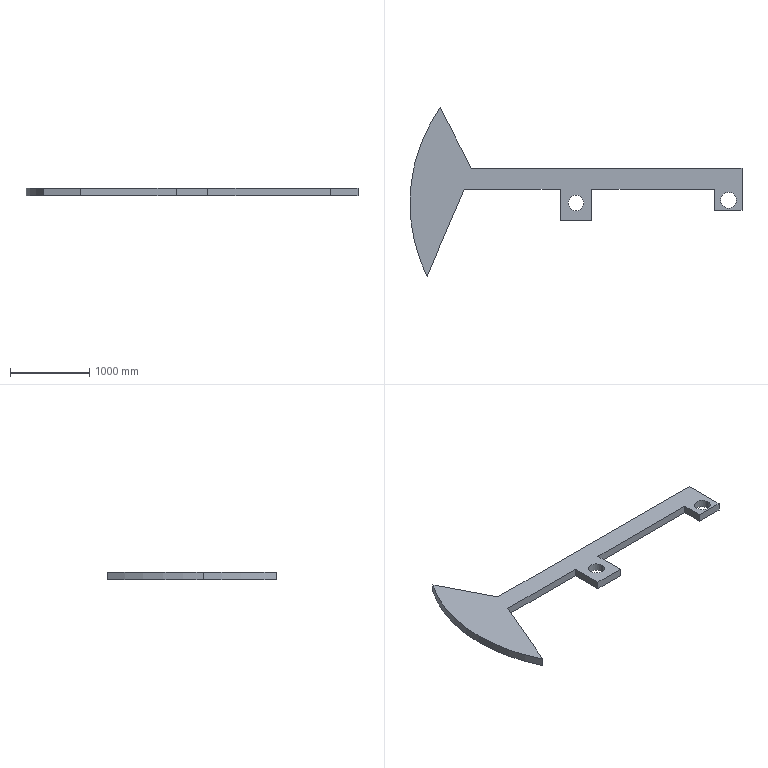Part | SolidWorks | features Extrusion 1, ICE 1 | 1 solid | 19 faces | box 4200 x 2133 x 100 mm | volume 203520372 mm3 | plane 13 | cylinder 6 | commonest cylinder face diameters 200 x4 4200 x2
STEP:
#1=CARTESIAN_POINT('',(-100.,0.,0.));
#2=VERTEX_POINT('',#1);
#3=CARTESIAN_POINT('',(100.,0.,0.));
#4=VERTEX_POINT('',#3);
#5=CARTESIAN_POINT('',(0.,0.,0.));
#6=DIRECTION('',(0.,0.,1.));
#7=DIRECTION('',(1.,0.,0.));
#8=AXIS2_PLACEMENT_3D('',#5,#6,#7);
#9=CIRCLE('',#8,100.);
#10=EDGE_CURVE('',#2,#4,#9,.T.);
#11=ORIENTED_EDGE('',*,*,#10,.F.);
#12=CARTESIAN_POINT('',(-100.,0.,100.));
#13=VERTEX_POINT('',#12);
#14=CARTESIAN_POINT('',(-100.,0.,0.));
#15=DIRECTION('',(0.,0.,1.));
#16=VECTOR('',#15,1000.);
#17=LINE('',#14,#16);
#18=EDGE_CURVE('',#2,#13,#17,.T.);
#19=ORIENTED_EDGE('',*,*,#18,.T.);
#20=CARTESIAN_POINT('',(100.,0.,100.));
#21=VERTEX_POINT('',#20);
#22=CARTESIAN_POINT('',(0.,0.,100.));
#23=DIRECTION('',(0.,0.,1.));
#24=DIRECTION('',(1.,0.,0.));
#25=AXIS2_PLACEMENT_3D('',#22,#23,#24);
#26=CIRCLE('',#25,100.);
#27=EDGE_CURVE('',#13,#21,#26,.T.);
#28=ORIENTED_EDGE('',*,*,#27,.T.);
#29=CARTESIAN_POINT('',(100.,0.,0.));
#30=DIRECTION('',(0.,0.,1.));
#31=VECTOR('',#30,1000.);
#32=LINE('',#29,#31);
#33=EDGE_CURVE('',#4,#21,#32,.T.);
#34=ORIENTED_EDGE('',*,*,#33,.F.);
#35=EDGE_LOOP('',(#11,#19,#28,#34));
#36=FACE_OUTER_BOUND('',#35,.T.);
#37=CARTESIAN_POINT('',(0.,0.,0.));
#38=DIRECTION('',(0.,0.,1.));
#39=DIRECTION('',(1.,0.,0.));
#40=AXIS2_PLACEMENT_3D('',#37,#38,#39);
#41=CYLINDRICAL_SURFACE('',#40,100.);
#42=ADVANCED_FACE('',(#36),#41,.F.);
#43=CARTESIAN_POINT('',(1830.038,35.754,0.));
#44=VERTEX_POINT('',#43);
#45=CARTESIAN_POINT('',(2030.038,35.754,0.));
#46=VERTEX_POINT('',#45);
#47=CARTESIAN_POINT('',(1930.038,35.754,0.));
#48=DIRECTION('',(0.,0.,1.));
#49=DIRECTION('',(1.,0.,0.));
#50=AXIS2_PLACEMENT_3D('',#47,#48,#49);
#51=CIRCLE('',#50,100.);
#52=EDGE_CURVE('',#44,#46,#51,.T.);
#53=ORIENTED_EDGE('',*,*,#52,.F.);
#54=CARTESIAN_POINT('',(1830.038,35.754,100.));
#55=VERTEX_POINT('',#54);
#56=CARTESIAN_POINT('',(1830.038,35.754,0.));
#57=DIRECTION('',(0.,0.,1.));
#58=VECTOR('',#57,1000.);
#59=LINE('',#56,#58);
#60=EDGE_CURVE('',#44,#55,#59,.T.);
#61=ORIENTED_EDGE('',*,*,#60,.T.);
#62=CARTESIAN_POINT('',(2030.038,35.754,100.));
#63=VERTEX_POINT('',#62);
#64=CARTESIAN_POINT('',(1930.038,35.754,100.));
#65=DIRECTION('',(0.,0.,1.));
#66=DIRECTION('',(1.,0.,0.));
#67=AXIS2_PLACEMENT_3D('',#64,#65,#66);
#68=CIRCLE('',#67,100.);
#69=EDGE_CURVE('',#55,#63,#68,.T.);
#70=ORIENTED_EDGE('',*,*,#69,.T.);
#71=CARTESIAN_POINT('',(2030.038,35.754,0.));
#72=DIRECTION('',(0.,0.,1.));
#73=VECTOR('',#72,1000.);
#74=LINE('',#71,#73);
#75=EDGE_CURVE('',#46,#63,#74,.T.);
#76=ORIENTED_EDGE('',*,*,#75,.F.);
#77=EDGE_LOOP('',(#53,#61,#70,#76));
#78=FACE_OUTER_BOUND('',#77,.T.);
#79=CARTESIAN_POINT('',(1930.038,35.754,0.));
#80=DIRECTION('',(0.,0.,1.));
#81=DIRECTION('',(1.,0.,0.));
#82=AXIS2_PLACEMENT_3D('',#79,#80,#81);
#83=CYLINDRICAL_SURFACE('',#82,100.);
#84=ADVANCED_FACE('',(#78),#83,.F.);
#85=CARTESIAN_POINT('',(-2100.,0.,100.));
#86=VERTEX_POINT('',#85);
#87=CARTESIAN_POINT('',(-1884.738,-926.156,100.));
#88=VERTEX_POINT('',#87);
#89=CARTESIAN_POINT('',(0.,0.,100.));
#90=DIRECTION('',(0.,0.,1.));
#91=DIRECTION('',(1.,0.,0.));
#92=AXIS2_PLACEMENT_3D('',#89,#90,#91);
#93=CIRCLE('',#92,2100.);
#94=EDGE_CURVE('',#86,#88,#93,.T.);
#95=ORIENTED_EDGE('',*,*,#94,.F.);
#96=CARTESIAN_POINT('',(-2100.,0.,0.));
#97=VERTEX_POINT('',#96);
#98=CARTESIAN_POINT('',(-2100.,0.,100.));
#99=DIRECTION('',(0.,0.,-1.));
#100=VECTOR('',#99,1000.);
#101=LINE('',#98,#100);
#102=EDGE_CURVE('',#86,#97,#101,.T.);
#103=ORIENTED_EDGE('',*,*,#102,.T.);
#104=CARTESIAN_POINT('',(-1884.738,-926.156,0.));
#105=VERTEX_POINT('',#104);
#106=CARTESIAN_POINT('',(0.,0.,0.));
#107=DIRECTION('',(0.,0.,1.));
#108=DIRECTION('',(1.,0.,0.));
#109=AXIS2_PLACEMENT_3D('',#106,#107,#108);
#110=CIRCLE('',#109,2100.);
#111=EDGE_CURVE('',#97,#105,#110,.T.);
#112=ORIENTED_EDGE('',*,*,#111,.T.);
#113=CARTESIAN_POINT('',(-1884.738,-926.156,100.));
#114=DIRECTION('',(0.,0.,-1.));
#115=VECTOR('',#114,1000.);
#116=LINE('',#113,#115);
#117=EDGE_CURVE('',#88,#105,#116,.T.);
#118=ORIENTED_EDGE('',*,*,#117,.F.);
#119=EDGE_LOOP('',(#95,#103,#112,#118));
#120=FACE_OUTER_BOUND('',#119,.T.);
#121=CARTESIAN_POINT('',(0.,0.,100.));
#122=DIRECTION('',(0.,0.,-1.));
#123=DIRECTION('',(-1.,0.,0.));
#124=AXIS2_PLACEMENT_3D('',#121,#122,#123);
#125=CYLINDRICAL_SURFACE('',#124,2100.);
#126=ADVANCED_FACE('',(#120),#125,.T.);
#127=CARTESIAN_POINT('',(-1322.571,440.167,0.));
#128=VERTEX_POINT('',#127);
#129=CARTESIAN_POINT('',(2100.,440.167,0.));
#130=VERTEX_POINT('',#129);
#131=CARTESIAN_POINT('',(-1322.571,440.167,0.));
#132=DIRECTION('',(1.,0.,0.));
#133=VECTOR('',#132,1000.);
#134=LINE('',#131,#133);
#135=EDGE_CURVE('',#128,#130,#134,.T.);
#136=ORIENTED_EDGE('',*,*,#135,.F.);
#137=CARTESIAN_POINT('',(-1322.571,440.167,100.));
#138=VERTEX_POINT('',#137);
#139=CARTESIAN_POINT('',(-1322.571,440.167,100.));
#140=DIRECTION('',(0.,0.,-1.));
#141=VECTOR('',#140,1000.);
#142=LINE('',#139,#141);
#143=EDGE_CURVE('',#138,#128,#142,.T.);
#144=ORIENTED_EDGE('',*,*,#143,.F.);
#145=CARTESIAN_POINT('',(2100.,440.167,100.));
#146=VERTEX_POINT('',#145);
#147=CARTESIAN_POINT('',(-1322.571,440.167,100.));
#148=DIRECTION('',(1.,0.,0.));
#149=VECTOR('',#148,1000.);
#150=LINE('',#147,#149);
#151=EDGE_CURVE('',#138,#146,#150,.T.);
#152=ORIENTED_EDGE('',*,*,#151,.T.);
#153=CARTESIAN_POINT('',(2100.,440.167,100.));
#154=DIRECTION('',(0.,0.,-1.));
#155=VECTOR('',#154,1000.);
#156=LINE('',#153,#155);
#157=EDGE_CURVE('',#146,#130,#156,.T.);
#158=ORIENTED_EDGE('',*,*,#157,.T.);
#159=EDGE_LOOP('',(#136,#144,#152,#158));
#160=FACE_OUTER_BOUND('',#159,.T.);
#161=CARTESIAN_POINT('',(-1322.571,440.167,100.));
#162=DIRECTION('',(0.,1.,0.));
#163=DIRECTION('',(0.,0.,1.));
#164=AXIS2_PLACEMENT_3D('',#161,#162,#163);
#165=PLANE('',#164);
#166=ADVANCED_FACE('',(#160),#165,.T.);
#167=CARTESIAN_POINT('',(-1718.675,1206.713,0.));
#168=VERTEX_POINT('',#167);
#169=CARTESIAN_POINT('',(-1718.675,1206.713,0.));
#170=DIRECTION('',(0.4591,-0.8884,0.));
#171=VECTOR('',#170,1000.);
#172=LINE('',#169,#171);
#173=EDGE_CURVE('',#168,#128,#172,.T.);
#174=ORIENTED_EDGE('',*,*,#173,.F.);
#175=CARTESIAN_POINT('',(-1718.675,1206.713,100.));
#176=VERTEX_POINT('',#175);
#177=CARTESIAN_POINT('',(-1718.675,1206.713,100.));
#178=DIRECTION('',(0.,0.,-1.));
#179=VECTOR('',#178,1000.);
#180=LINE('',#177,#179);
#181=EDGE_CURVE('',#176,#168,#180,.T.);
#182=ORIENTED_EDGE('',*,*,#181,.F.);
#183=CARTESIAN_POINT('',(-1718.675,1206.713,100.));
#184=DIRECTION('',(0.4591,-0.8884,0.));
#185=VECTOR('',#184,1000.);
#186=LINE('',#183,#185);
#187=EDGE_CURVE('',#176,#138,#186,.T.);
#188=ORIENTED_EDGE('',*,*,#187,.T.);
#189=ORIENTED_EDGE('',*,*,#143,.T.);
#190=EDGE_LOOP('',(#174,#182,#188,#189));
#191=FACE_OUTER_BOUND('',#190,.T.);
#192=CARTESIAN_POINT('',(-1718.675,1206.713,100.));
#193=DIRECTION('',(0.8884,0.4591,0.));
#194=DIRECTION('',(-0.4591,0.8884,0.));
#195=AXIS2_PLACEMENT_3D('',#192,#193,#194);
#196=PLANE('',#195);
#197=ADVANCED_FACE('',(#191),#196,.T.);
#198=ORIENTED_EDGE('',*,*,#102,.F.);
#199=CARTESIAN_POINT('',(0.,0.,100.));
#200=DIRECTION('',(0.,0.,1.));
#201=DIRECTION('',(1.,0.,0.));
#202=AXIS2_PLACEMENT_3D('',#199,#200,#201);
#203=CIRCLE('',#202,2100.);
#204=EDGE_CURVE('',#176,#86,#203,.T.);
#205=ORIENTED_EDGE('',*,*,#204,.F.);
#206=ORIENTED_EDGE('',*,*,#181,.T.);
#207=CARTESIAN_POINT('',(0.,0.,0.));
#208=DIRECTION('',(0.,0.,1.));
#209=DIRECTION('',(1.,0.,0.));
#210=AXIS2_PLACEMENT_3D('',#207,#208,#209);
#211=CIRCLE('',#210,2100.);
#212=EDGE_CURVE('',#168,#97,#211,.T.);
#213=ORIENTED_EDGE('',*,*,#212,.T.);
#214=EDGE_LOOP('',(#198,#205,#206,#213));
#215=FACE_OUTER_BOUND('',#214,.T.);
#216=CARTESIAN_POINT('',(0.,0.,100.));
#217=DIRECTION('',(0.,0.,-1.));
#218=DIRECTION('',(-1.,0.,0.));
#219=AXIS2_PLACEMENT_3D('',#216,#217,#218);
#220=CYLINDRICAL_SURFACE('',#219,2100.);
#221=ADVANCED_FACE('',(#215),#220,.T.);
#222=CARTESIAN_POINT('',(-1413.953,173.884,0.));
#223=VERTEX_POINT('',#222);
#224=CARTESIAN_POINT('',(-1884.738,-926.156,0.));
#225=DIRECTION('',(0.3935,0.9193,0.));
#226=VECTOR('',#225,1000.);
#227=LINE('',#224,#226);
#228=EDGE_CURVE('',#105,#223,#227,.T.);
#229=ORIENTED_EDGE('',*,*,#228,.T.);
#230=CARTESIAN_POINT('',(-1413.953,173.884,100.));
#231=VERTEX_POINT('',#230);
#232=CARTESIAN_POINT('',(-1413.953,173.884,100.));
#233=DIRECTION('',(0.,0.,-1.));
#234=VECTOR('',#233,1000.);
#235=LINE('',#232,#234);
#236=EDGE_CURVE('',#231,#223,#235,.T.);
#237=ORIENTED_EDGE('',*,*,#236,.F.);
#238=CARTESIAN_POINT('',(-1884.738,-926.156,100.));
#239=DIRECTION('',(0.3935,0.9193,0.));
#240=VECTOR('',#239,1000.);
#241=LINE('',#238,#240);
#242=EDGE_CURVE('',#88,#231,#241,.T.);
#243=ORIENTED_EDGE('',*,*,#242,.F.);
#244=ORIENTED_EDGE('',*,*,#117,.T.);
#245=EDGE_LOOP('',(#229,#237,#243,#244));
#246=FACE_OUTER_BOUND('',#245,.T.);
#247=CARTESIAN_POINT('',(-1884.738,-926.156,100.));
#248=DIRECTION('',(-0.9193,0.3935,0.));
#249=DIRECTION('',(-0.3935,-0.9193,0.));
#250=AXIS2_PLACEMENT_3D('',#247,#248,#249);
#251=PLANE('',#250);
#252=ADVANCED_FACE('',(#246),#251,.F.);
#253=CARTESIAN_POINT('',(-200.,173.884,0.));
#254=VERTEX_POINT('',#253);
#255=CARTESIAN_POINT('',(-1413.953,173.884,0.));
#256=DIRECTION('',(1.,0.,0.));
#257=VECTOR('',#256,1000.);
#258=LINE('',#255,#257);
#259=EDGE_CURVE('',#223,#254,#258,.T.);
#260=ORIENTED_EDGE('',*,*,#259,.T.);
#261=CARTESIAN_POINT('',(-200.,173.884,100.));
#262=VERTEX_POINT('',#261);
#263=CARTESIAN_POINT('',(-200.,173.884,100.));
#264=DIRECTION('',(0.,0.,-1.));
#265=VECTOR('',#264,1000.);
#266=LINE('',#263,#265);
#267=EDGE_CURVE('',#262,#254,#266,.T.);
#268=ORIENTED_EDGE('',*,*,#267,.F.);
#269=CARTESIAN_POINT('',(-1413.953,173.884,100.));
#270=DIRECTION('',(1.,0.,0.));
#271=VECTOR('',#270,1000.);
#272=LINE('',#269,#271);
#273=EDGE_CURVE('',#231,#262,#272,.T.);
#274=ORIENTED_EDGE('',*,*,#273,.F.);
#275=ORIENTED_EDGE('',*,*,#236,.T.);
#276=EDGE_LOOP('',(#260,#268,#274,#275));
#277=FACE_OUTER_BOUND('',#276,.T.);
#278=CARTESIAN_POINT('',(-1413.953,173.884,100.));
#279=DIRECTION('',(0.,1.,0.));
#280=DIRECTION('',(0.,0.,1.));
#281=AXIS2_PLACEMENT_3D('',#278,#279,#280);
#282=PLANE('',#281);
#283=ADVANCED_FACE('',(#277),#282,.F.);
#284=CARTESIAN_POINT('',(-200.,-226.116,0.));
#285=VERTEX_POINT('',#284);
#286=CARTESIAN_POINT('',(-200.,173.884,0.));
#287=DIRECTION('',(0.,-1.,0.));
#288=VECTOR('',#287,1000.);
#289=LINE('',#286,#288);
#290=EDGE_CURVE('',#254,#285,#289,.T.);
#291=ORIENTED_EDGE('',*,*,#290,.T.);
#292=CARTESIAN_POINT('',(-200.,-226.116,100.));
#293=VERTEX_POINT('',#292);
#294=CARTESIAN_POINT('',(-200.,-226.116,100.));
#295=DIRECTION('',(0.,0.,-1.));
#296=VECTOR('',#295,1000.);
#297=LINE('',#294,#296);
#298=EDGE_CURVE('',#293,#285,#297,.T.);
#299=ORIENTED_EDGE('',*,*,#298,.F.);
#300=CARTESIAN_POINT('',(-200.,173.884,100.));
#301=DIRECTION('',(0.,-1.,0.));
#302=VECTOR('',#301,1000.);
#303=LINE('',#300,#302);
#304=EDGE_CURVE('',#262,#293,#303,.T.);
#305=ORIENTED_EDGE('',*,*,#304,.F.);
#306=ORIENTED_EDGE('',*,*,#267,.T.);
#307=EDGE_LOOP('',(#291,#299,#305,#306));
#308=FACE_OUTER_BOUND('',#307,.T.);
#309=CARTESIAN_POINT('',(-200.,173.884,100.));
#310=DIRECTION('',(1.,0.,0.));
#311=DIRECTION('',(0.,1.,0.));
#312=AXIS2_PLACEMENT_3D('',#309,#310,#311);
#313=PLANE('',#312);
#314=ADVANCED_FACE('',(#308),#313,.F.);
#315=CARTESIAN_POINT('',(200.,-226.116,0.));
#316=VERTEX_POINT('',#315);
#317=CARTESIAN_POINT('',(-200.,-226.116,0.));
#318=DIRECTION('',(1.,0.,0.));
#319=VECTOR('',#318,1000.);
#320=LINE('',#317,#319);
#321=EDGE_CURVE('',#285,#316,#320,.T.);
#322=ORIENTED_EDGE('',*,*,#321,.T.);
#323=CARTESIAN_POINT('',(200.,-226.116,100.));
#324=VERTEX_POINT('',#323);
#325=CARTESIAN_POINT('',(200.,-226.116,100.));
#326=DIRECTION('',(0.,0.,-1.));
#327=VECTOR('',#326,1000.);
#328=LINE('',#325,#327);
#329=EDGE_CURVE('',#324,#316,#328,.T.);
#330=ORIENTED_EDGE('',*,*,#329,.F.);
#331=CARTESIAN_POINT('',(-200.,-226.116,100.));
#332=DIRECTION('',(1.,0.,0.));
#333=VECTOR('',#332,1000.);
#334=LINE('',#331,#333);
#335=EDGE_CURVE('',#293,#324,#334,.T.);
#336=ORIENTED_EDGE('',*,*,#335,.F.);
#337=ORIENTED_EDGE('',*,*,#298,.T.);
#338=EDGE_LOOP('',(#322,#330,#336,#337));
#339=FACE_OUTER_BOUND('',#338,.T.);
#340=CARTESIAN_POINT('',(-200.,-226.116,100.));
#341=DIRECTION('',(0.,1.,0.));
#342=DIRECTION('',(0.,0.,1.));
#343=AXIS2_PLACEMENT_3D('',#340,#341,#342);
#344=PLANE('',#343);
#345=ADVANCED_FACE('',(#339),#344,.F.);
#346=CARTESIAN_POINT('',(200.,173.884,0.));
#347=VERTEX_POINT('',#346);
#348=CARTESIAN_POINT('',(200.,-226.116,0.));
#349=DIRECTION('',(0.,1.,0.));
#350=VECTOR('',#349,1000.);
#351=LINE('',#348,#350);
#352=EDGE_CURVE('',#316,#347,#351,.T.);
#353=ORIENTED_EDGE('',*,*,#352,.T.);
#354=CARTESIAN_POINT('',(200.,173.884,100.));
#355=VERTEX_POINT('',#354);
#356=CARTESIAN_POINT('',(200.,173.884,100.));
#357=DIRECTION('',(0.,0.,-1.));
#358=VECTOR('',#357,1000.);
#359=LINE('',#356,#358);
#360=EDGE_CURVE('',#355,#347,#359,.T.);
#361=ORIENTED_EDGE('',*,*,#360,.F.);
#362=CARTESIAN_POINT('',(200.,-226.116,100.));
#363=DIRECTION('',(0.,1.,0.));
#364=VECTOR('',#363,1000.);
#365=LINE('',#362,#364);
#366=EDGE_CURVE('',#324,#355,#365,.T.);
#367=ORIENTED_EDGE('',*,*,#366,.F.);
#368=ORIENTED_EDGE('',*,*,#329,.T.);
#369=EDGE_LOOP('',(#353,#361,#367,#368));
#370=FACE_OUTER_BOUND('',#369,.T.);
#371=CARTESIAN_POINT('',(200.,-226.116,100.));
#372=DIRECTION('',(-1.,0.,0.));
#373=DIRECTION('',(0.,0.,1.));
#374=AXIS2_PLACEMENT_3D('',#371,#372,#373);
#375=PLANE('',#374);
#376=ADVANCED_FACE('',(#370),#375,.F.);
#377=CARTESIAN_POINT('',(1753.895,173.884,0.));
#378=VERTEX_POINT('',#377);
#379=CARTESIAN_POINT('',(1098.892,173.884,0.));
#380=DIRECTION('',(1.,0.,0.));
#381=VECTOR('',#380,1000.);
#382=LINE('',#379,#381);
#383=EDGE_CURVE('',#347,#378,#382,.T.);
#384=ORIENTED_EDGE('',*,*,#383,.T.);
#385=CARTESIAN_POINT('',(1753.895,173.884,100.));
#386=VERTEX_POINT('',#385);
#387=CARTESIAN_POINT('',(1753.895,173.884,100.));
#388=DIRECTION('',(0.,0.,-1.));
#389=VECTOR('',#388,1000.);
#390=LINE('',#387,#389);
#391=EDGE_CURVE('',#386,#378,#390,.T.);
#392=ORIENTED_EDGE('',*,*,#391,.F.);
#393=CARTESIAN_POINT('',(200.,173.884,100.));
#394=DIRECTION('',(1.,0.,0.));
#395=VECTOR('',#394,1000.);
#396=LINE('',#393,#395);
#397=EDGE_CURVE('',#355,#386,#396,.T.);
#398=ORIENTED_EDGE('',*,*,#397,.F.);
#399=ORIENTED_EDGE('',*,*,#360,.T.);
#400=EDGE_LOOP('',(#384,#392,#398,#399));
#401=FACE_OUTER_BOUND('',#400,.T.);
#402=CARTESIAN_POINT('',(1098.892,173.884,100.));
#403=DIRECTION('',(0.,1.,0.));
#404=DIRECTION('',(0.,0.,1.));
#405=AXIS2_PLACEMENT_3D('',#402,#403,#404);
#406=PLANE('',#405);
#407=ADVANCED_FACE('',(#401),#406,.F.);
#408=CARTESIAN_POINT('',(1753.895,-92.399,0.));
#409=VERTEX_POINT('',#408);
#410=CARTESIAN_POINT('',(1753.895,173.884,0.));
#411=DIRECTION('',(0.,-1.,0.));
#412=VECTOR('',#411,1000.);
#413=LINE('',#410,#412);
#414=EDGE_CURVE('',#378,#409,#413,.T.);
#415=ORIENTED_EDGE('',*,*,#414,.T.);
#416=CARTESIAN_POINT('',(1753.895,-92.399,100.));
#417=VERTEX_POINT('',#416);
#418=CARTESIAN_POINT('',(1753.895,-92.399,100.));
#419=DIRECTION('',(0.,0.,-1.));
#420=VECTOR('',#419,1000.);
#421=LINE('',#418,#420);
#422=EDGE_CURVE('',#417,#409,#421,.T.);
#423=ORIENTED_EDGE('',*,*,#422,.F.);
#424=CARTESIAN_POINT('',(1753.895,173.884,100.));
#425=DIRECTION('',(0.,-1.,0.));
#426=VECTOR('',#425,1000.);
#427=LINE('',#424,#426);
#428=EDGE_CURVE('',#386,#417,#427,.T.);
#429=ORIENTED_EDGE('',*,*,#428,.F.);
#430=ORIENTED_EDGE('',*,*,#391,.T.);
#431=EDGE_LOOP('',(#415,#423,#429,#430));
#432=FACE_OUTER_BOUND('',#431,.T.);
#433=CARTESIAN_POINT('',(1753.895,173.884,100.));
#434=DIRECTION('',(1.,0.,0.));
#435=DIRECTION('',(0.,0.,-1.));
#436=AXIS2_PLACEMENT_3D('',#433,#434,#435);
#437=PLANE('',#436);
#438=ADVANCED_FACE('',(#432),#437,.F.);
#439=CARTESIAN_POINT('',(2100.,-92.399,0.));
#440=VERTEX_POINT('',#439);
#441=CARTESIAN_POINT('',(1753.895,-92.399,0.));
#442=DIRECTION('',(1.,0.,0.));
#443=VECTOR('',#442,1000.);
#444=LINE('',#441,#443);
#445=EDGE_CURVE('',#409,#440,#444,.T.);
#446=ORIENTED_EDGE('',*,*,#445,.T.);
#447=CARTESIAN_POINT('',(2100.,-92.399,100.));
#448=VERTEX_POINT('',#447);
#449=CARTESIAN_POINT('',(2100.,-92.399,100.));
#450=DIRECTION('',(0.,0.,-1.));
#451=VECTOR('',#450,1000.);
#452=LINE('',#449,#451);
#453=EDGE_CURVE('',#448,#440,#452,.T.);
#454=ORIENTED_EDGE('',*,*,#453,.F.);
#455=CARTESIAN_POINT('',(1753.895,-92.399,100.));
#456=DIRECTION('',(1.,0.,0.));
#457=VECTOR('',#456,1000.);
#458=LINE('',#455,#457);
#459=EDGE_CURVE('',#417,#448,#458,.T.);
#460=ORIENTED_EDGE('',*,*,#459,.F.);
#461=ORIENTED_EDGE('',*,*,#422,.T.);
#462=EDGE_LOOP('',(#446,#454,#460,#461));
#463=FACE_OUTER_BOUND('',#462,.T.);
#464=CARTESIAN_POINT('',(1753.895,-92.399,100.));
#465=DIRECTION('',(0.,1.,0.));
#466=DIRECTION('',(0.,0.,1.));
#467=AXIS2_PLACEMENT_3D('',#464,#465,#466);
#468=PLANE('',#467);
#469=ADVANCED_FACE('',(#463),#468,.F.);
#470=CARTESIAN_POINT('',(2100.,-92.399,0.));
#471=DIRECTION('',(0.,1.,0.));
#472=VECTOR('',#471,1000.);
#473=LINE('',#470,#472);
#474=EDGE_CURVE('',#440,#130,#473,.T.);
#475=ORIENTED_EDGE('',*,*,#474,.T.);
#476=ORIENTED_EDGE('',*,*,#157,.F.);
#477=CARTESIAN_POINT('',(2100.,173.884,100.));
#478=DIRECTION('',(0.,1.,0.));
#479=VECTOR('',#478,1000.);
#480=LINE('',#477,#479);
#481=EDGE_CURVE('',#448,#146,#480,.T.);
#482=ORIENTED_EDGE('',*,*,#481,.F.);
#483=ORIENTED_EDGE('',*,*,#453,.T.);
#484=EDGE_LOOP('',(#475,#476,#482,#483));
#485=FACE_OUTER_BOUND('',#484,.T.);
#486=CARTESIAN_POINT('',(2100.,-92.399,100.));
#487=DIRECTION('',(-1.,0.,0.));
#488=DIRECTION('',(0.,0.,1.));
#489=AXIS2_PLACEMENT_3D('',#486,#487,#488);
#490=PLANE('',#489);
#491=ADVANCED_FACE('',(#485),#490,.F.);
#492=CARTESIAN_POINT('',(0.,0.,100.));
#493=DIRECTION('',(0.,0.,1.));
#494=DIRECTION('',(1.,0.,0.));
#495=AXIS2_PLACEMENT_3D('',#492,#493,#494);
#496=CIRCLE('',#495,100.);
#497=EDGE_CURVE('',#21,#13,#496,.T.);
#498=ORIENTED_EDGE('',*,*,#497,.F.);
#499=ORIENTED_EDGE('',*,*,#27,.F.);
#500=EDGE_LOOP('',(#498,#499));
#501=FACE_BOUND('',#500,.T.);
#502=CARTESIAN_POINT('',(1930.038,35.754,100.));
#503=DIRECTION('',(0.,0.,1.));
#504=DIRECTION('',(1.,0.,0.));
#505=AXIS2_PLACEMENT_3D('',#502,#503,#504);
#506=CIRCLE('',#505,100.);
#507=EDGE_CURVE('',#63,#55,#506,.T.);
#508=ORIENTED_EDGE('',*,*,#507,.F.);
#509=ORIENTED_EDGE('',*,*,#69,.F.);
#510=EDGE_LOOP('',(#508,#509));
#511=FACE_BOUND('',#510,.T.);
#512=ORIENTED_EDGE('',*,*,#481,.T.);
#513=ORIENTED_EDGE('',*,*,#151,.F.);
#514=ORIENTED_EDGE('',*,*,#187,.F.);
#515=ORIENTED_EDGE('',*,*,#204,.T.);
#516=ORIENTED_EDGE('',*,*,#94,.T.);
#517=ORIENTED_EDGE('',*,*,#242,.T.);
#518=ORIENTED_EDGE('',*,*,#273,.T.);
#519=ORIENTED_EDGE('',*,*,#304,.T.);
#520=ORIENTED_EDGE('',*,*,#335,.T.);
#521=ORIENTED_EDGE('',*,*,#366,.T.);
#522=ORIENTED_EDGE('',*,*,#397,.T.);
#523=ORIENTED_EDGE('',*,*,#428,.T.);
#524=ORIENTED_EDGE('',*,*,#459,.T.);
#525=EDGE_LOOP('',(#512,#513,#514,#515,#516,#517,#518,#519,#520,#521,#522,#523,#524));
#526=FACE_OUTER_BOUND('',#525,.T.);
#527=CARTESIAN_POINT('',(0.,0.,100.));
#528=DIRECTION('',(0.,0.,1.));
#529=DIRECTION('',(1.,0.,0.));
#530=AXIS2_PLACEMENT_3D('',#527,#528,#529);
#531=PLANE('',#530);
#532=ADVANCED_FACE('',(#501,#511,#526),#531,.T.);
#533=CARTESIAN_POINT('',(0.,0.,0.));
#534=DIRECTION('',(0.,0.,1.));
#535=DIRECTION('',(1.,0.,0.));
#536=AXIS2_PLACEMENT_3D('',#533,#534,#535);
#537=CIRCLE('',#536,100.);
#538=EDGE_CURVE('',#4,#2,#537,.T.);
#539=ORIENTED_EDGE('',*,*,#538,.T.);
#540=ORIENTED_EDGE('',*,*,#10,.T.);
#541=EDGE_LOOP('',(#539,#540));
#542=FACE_BOUND('',#541,.T.);
#543=CARTESIAN_POINT('',(1930.038,35.754,0.));
#544=DIRECTION('',(0.,0.,1.));
#545=DIRECTION('',(1.,0.,0.));
#546=AXIS2_PLACEMENT_3D('',#543,#544,#545);
#547=CIRCLE('',#546,100.);
#548=EDGE_CURVE('',#46,#44,#547,.T.);
#549=ORIENTED_EDGE('',*,*,#548,.T.);
#550=ORIENTED_EDGE('',*,*,#52,.T.);
#551=EDGE_LOOP('',(#549,#550));
#552=FACE_BOUND('',#551,.T.);
#553=ORIENTED_EDGE('',*,*,#135,.T.);
#554=ORIENTED_EDGE('',*,*,#474,.F.);
#555=ORIENTED_EDGE('',*,*,#445,.F.);
#556=ORIENTED_EDGE('',*,*,#414,.F.);
#557=ORIENTED_EDGE('',*,*,#383,.F.);
#558=ORIENTED_EDGE('',*,*,#352,.F.);
#559=ORIENTED_EDGE('',*,*,#321,.F.);
#560=ORIENTED_EDGE('',*,*,#290,.F.);
#561=ORIENTED_EDGE('',*,*,#259,.F.);
#562=ORIENTED_EDGE('',*,*,#228,.F.);
#563=ORIENTED_EDGE('',*,*,#111,.F.);
#564=ORIENTED_EDGE('',*,*,#212,.F.);
#565=ORIENTED_EDGE('',*,*,#173,.T.);
#566=EDGE_LOOP('',(#553,#554,#555,#556,#557,#558,#559,#560,#561,#562,#563,#564,#565));
#567=FACE_OUTER_BOUND('',#566,.T.);
#568=CARTESIAN_POINT('',(0.,0.,0.));
#569=DIRECTION('',(0.,0.,1.));
#570=DIRECTION('',(1.,0.,0.));
#571=AXIS2_PLACEMENT_3D('',#568,#569,#570);
#572=PLANE('',#571);
#573=ADVANCED_FACE('',(#542,#552,#567),#572,.F.);
#574=ORIENTED_EDGE('',*,*,#60,.F.);
#575=ORIENTED_EDGE('',*,*,#548,.F.);
#576=ORIENTED_EDGE('',*,*,#75,.T.);
#577=ORIENTED_EDGE('',*,*,#507,.T.);
#578=EDGE_LOOP('',(#574,#575,#576,#577));
#579=FACE_OUTER_BOUND('',#578,.T.);
#580=CARTESIAN_POINT('',(1930.038,35.754,0.));
#581=DIRECTION('',(0.,0.,1.));
#582=DIRECTION('',(1.,0.,0.));
#583=AXIS2_PLACEMENT_3D('',#580,#581,#582);
#584=CYLINDRICAL_SURFACE('',#583,100.);
#585=ADVANCED_FACE('',(#579),#584,.F.);
#586=ORIENTED_EDGE('',*,*,#18,.F.);
#587=ORIENTED_EDGE('',*,*,#538,.F.);
#588=ORIENTED_EDGE('',*,*,#33,.T.);
#589=ORIENTED_EDGE('',*,*,#497,.T.);
#590=EDGE_LOOP('',(#586,#587,#588,#589));
#591=FACE_OUTER_BOUND('',#590,.T.);
#592=CARTESIAN_POINT('',(0.,0.,0.));
#593=DIRECTION('',(0.,0.,1.));
#594=DIRECTION('',(1.,0.,0.));
#595=AXIS2_PLACEMENT_3D('',#592,#593,#594);
#596=CYLINDRICAL_SURFACE('',#595,100.);
#597=ADVANCED_FACE('',(#591),#596,.F.);
#598=CLOSED_SHELL('',(#42,#84,#126,#166,#197,#221,#252,#283,#314,#345,#376,#407,#438,#469,#491,#532,#573,#585,#597));
#599=MANIFOLD_SOLID_BREP('',#598);
#600=CARTESIAN_POINT('',(0.,0.,0.));
#601=DIRECTION('',(0.,0.,1.));
#602=DIRECTION('',(1.,0.,0.));
#603=AXIS2_PLACEMENT_3D('',#600,#601,#602);
#604=(LENGTH_UNIT()NAMED_UNIT(*)SI_UNIT(.MILLI.,.METRE.));
#605=UNCERTAINTY_MEASURE_WITH_UNIT(LENGTH_MEASURE(0.00001),#604,'','');
#606=(NAMED_UNIT(*)PLANE_ANGLE_UNIT()SI_UNIT($,.RADIAN.));
#607=(NAMED_UNIT(*)SI_UNIT($,.STERADIAN.)SOLID_ANGLE_UNIT());
#608=(GEOMETRIC_REPRESENTATION_CONTEXT(3)GLOBAL_UNCERTAINTY_ASSIGNED_CONTEXT((#605))GLOBAL_UNIT_ASSIGNED_CONTEXT((#604,#606,#607))REPRESENTATION_CONTEXT('',''));
#609=ADVANCED_BREP_SHAPE_REPRESENTATION('',(#599,#603),#608);